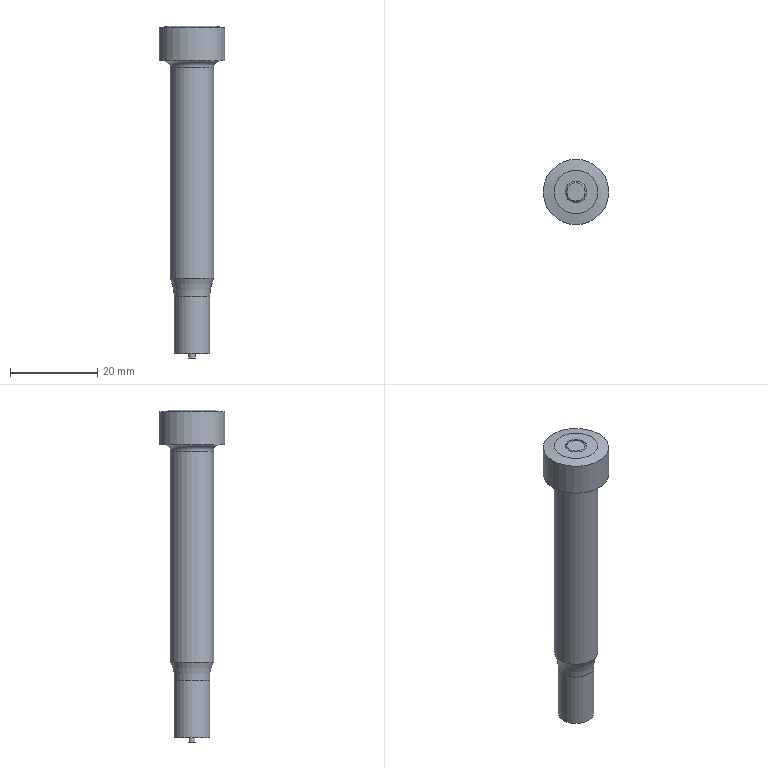Part | NX | features APJAS10-90-P8.10_2 2 | 1 solid | 20 faces | box 15 x 15 x 76 mm | volume 6168 mm3 | cylinder 8 | plane 7 | torus 2 | cone 2 | spline 1 | commonest cylinder face diameters 1.6 x1 1.8 x1 4.2 x1 4.4 x1 4.9 x1 8.1 x1
STEP:
#1=CARTESIAN_POINT('',(-219.,86.,60.5));
#2=VERTEX_POINT('',#1);
#3=CARTESIAN_POINT('',(-214.,86.,60.5));
#4=DIRECTION('',(0.,0.,1.));
#5=DIRECTION('',(1.,0.,0.));
#6=AXIS2_PLACEMENT_3D('',#3,#4,#5);
#7=CIRCLE('',#6,5.);
#8=EDGE_CURVE('',#2,#2,#7,.T.);
#9=ORIENTED_EDGE('',*,*,#8,.F.);
#10=EDGE_LOOP('',(#9));
#11=FACE_BOUND('',#10,.T.);
#12=CARTESIAN_POINT('',(-209.,86.,12.254));
#13=VERTEX_POINT('',#12);
#14=CARTESIAN_POINT('',(-214.,86.,12.254));
#15=DIRECTION('',(0.,0.,1.));
#16=DIRECTION('',(-1.,0.,0.));
#17=AXIS2_PLACEMENT_3D('',#14,#15,#16);
#18=CIRCLE('',#17,5.);
#19=EDGE_CURVE('',#13,#13,#18,.T.);
#20=ORIENTED_EDGE('',*,*,#19,.T.);
#21=EDGE_LOOP('',(#20));
#22=FACE_BOUND('',#21,.T.);
#23=CARTESIAN_POINT('',(-214.,86.,42.5));
#24=DIRECTION('',(0.,0.,-1.));
#25=DIRECTION('',(1.,0.,0.));
#26=AXIS2_PLACEMENT_3D('',#23,#24,#25);
#27=CYLINDRICAL_SURFACE('',#26,5.);
#28=ADVANCED_FACE('',(#11,#22),#27,.T.);
#29=CARTESIAN_POINT('',(-214.9,86.,23.));
#30=VERTEX_POINT('',#29);
#31=CARTESIAN_POINT('',(-214.,86.,23.));
#32=DIRECTION('',(0.,0.,1.));
#33=DIRECTION('',(-1.,0.,0.));
#34=AXIS2_PLACEMENT_3D('',#31,#32,#33);
#35=CIRCLE('',#34,0.9);
#36=EDGE_CURVE('',#30,#30,#35,.T.);
#37=ORIENTED_EDGE('',*,*,#36,.T.);
#38=EDGE_LOOP('',(#37));
#39=FACE_BOUND('',#38,.T.);
#40=CARTESIAN_POINT('',(-214.9,86.,-5.));
#41=VERTEX_POINT('',#40);
#42=CARTESIAN_POINT('',(-214.,86.,-5.));
#43=DIRECTION('',(0.,0.,1.));
#44=DIRECTION('',(-1.,0.,0.));
#45=AXIS2_PLACEMENT_3D('',#42,#43,#44);
#46=CIRCLE('',#45,0.9);
#47=EDGE_CURVE('',#41,#41,#46,.T.);
#48=ORIENTED_EDGE('',*,*,#47,.F.);
#49=EDGE_LOOP('',(#48));
#50=FACE_BOUND('',#49,.T.);
#51=CARTESIAN_POINT('',(-214.,86.,9.));
#52=DIRECTION('',(0.,0.,-1.));
#53=DIRECTION('',(1.,0.,0.));
#54=AXIS2_PLACEMENT_3D('',#51,#52,#53);
#55=CYLINDRICAL_SURFACE('',#54,0.9);
#56=ADVANCED_FACE('',(#39,#50),#55,.F.);
#57=CARTESIAN_POINT('',(-211.55,86.,69.632));
#58=VERTEX_POINT('',#57);
#59=CARTESIAN_POINT('',(-214.,86.,69.632));
#60=DIRECTION('',(0.,0.,1.));
#61=DIRECTION('',(1.,0.,0.));
#62=AXIS2_PLACEMENT_3D('',#59,#60,#61);
#63=CIRCLE('',#62,2.45);
#64=EDGE_CURVE('',#58,#58,#63,.T.);
#65=ORIENTED_EDGE('',*,*,#64,.F.);
#66=EDGE_LOOP('',(#65));
#67=FACE_BOUND('',#66,.T.);
#68=CARTESIAN_POINT('',(-216.45,86.,70.));
#69=VERTEX_POINT('',#68);
#70=CARTESIAN_POINT('',(-214.,86.,70.));
#71=DIRECTION('',(0.,0.,-1.));
#72=DIRECTION('',(-1.,0.,0.));
#73=AXIS2_PLACEMENT_3D('',#70,#71,#72);
#74=CIRCLE('',#73,2.45);
#75=EDGE_CURVE('',#69,#69,#74,.T.);
#76=ORIENTED_EDGE('',*,*,#75,.F.);
#77=EDGE_LOOP('',(#76));
#78=FACE_BOUND('',#77,.T.);
#79=CARTESIAN_POINT('',(-214.,86.,68.775));
#80=DIRECTION('',(0.,0.,-1.));
#81=DIRECTION('',(1.,0.,0.));
#82=AXIS2_PLACEMENT_3D('',#79,#80,#81);
#83=CYLINDRICAL_SURFACE('',#82,2.45);
#84=ADVANCED_FACE('',(#67,#78),#83,.F.);
#85=ORIENTED_EDGE('',*,*,#8,.T.);
#86=EDGE_LOOP('',(#85));
#87=FACE_BOUND('',#86,.T.);
#88=CARTESIAN_POINT('',(-220.5,86.,62.));
#89=VERTEX_POINT('',#88);
#90=CARTESIAN_POINT('',(-214.,86.,62.));
#91=DIRECTION('',(0.,0.,-1.));
#92=DIRECTION('',(1.,0.,0.));
#93=AXIS2_PLACEMENT_3D('',#90,#91,#92);
#94=CIRCLE('',#93,6.5);
#95=EDGE_CURVE('',#89,#89,#94,.T.);
#96=ORIENTED_EDGE('',*,*,#95,.T.);
#97=EDGE_LOOP('',(#96));
#98=FACE_BOUND('',#97,.T.);
#99=CARTESIAN_POINT('',(-214.,86.,60.5));
#100=DIRECTION('',(0.,0.,1.));
#101=DIRECTION('',(-1.,0.,0.));
#102=AXIS2_PLACEMENT_3D('',#99,#100,#101);
#103=TOROIDAL_SURFACE('',#102,6.5,1.5);
#104=ADVANCED_FACE('',(#87,#98),#103,.F.);
#105=CARTESIAN_POINT('',(-221.5,86.,62.));
#106=VERTEX_POINT('',#105);
#107=CARTESIAN_POINT('',(-214.,86.,62.));
#108=DIRECTION('',(0.,0.,-1.));
#109=DIRECTION('',(-1.,0.,0.));
#110=AXIS2_PLACEMENT_3D('',#107,#108,#109);
#111=CIRCLE('',#110,7.5);
#112=EDGE_CURVE('',#106,#106,#111,.T.);
#113=ORIENTED_EDGE('',*,*,#112,.T.);
#114=EDGE_LOOP('',(#113));
#115=FACE_BOUND('',#114,.T.);
#116=ORIENTED_EDGE('',*,*,#95,.F.);
#117=EDGE_LOOP('',(#116));
#118=FACE_BOUND('',#117,.T.);
#119=CARTESIAN_POINT('',(-214.,86.,62.));
#120=DIRECTION('',(0.,0.,-1.));
#121=DIRECTION('',(1.,0.,0.));
#122=AXIS2_PLACEMENT_3D('',#119,#120,#121);
#123=PLANE('',#122);
#124=ADVANCED_FACE('',(#115,#118),#123,.T.);
#125=CARTESIAN_POINT('',(-218.05,86.,8.));
#126=VERTEX_POINT('',#125);
#127=CARTESIAN_POINT('',(-214.,86.,8.));
#128=DIRECTION('',(0.,0.,1.));
#129=DIRECTION('',(-1.,0.,0.));
#130=AXIS2_PLACEMENT_3D('',#127,#128,#129);
#131=CIRCLE('',#130,4.05);
#132=EDGE_CURVE('',#126,#126,#131,.T.);
#133=ORIENTED_EDGE('',*,*,#132,.T.);
#134=EDGE_LOOP('',(#133));
#135=FACE_BOUND('',#134,.T.);
#136=ORIENTED_EDGE('',*,*,#19,.F.);
#137=EDGE_LOOP('',(#136));
#138=FACE_BOUND('',#137,.T.);
#139=CARTESIAN_POINT('',(-214.,86.,8.));
#140=DIRECTION('',(0.,0.,-1.));
#141=DIRECTION('',(1.,0.,0.));
#142=AXIS2_PLACEMENT_3D('',#139,#140,#141);
#143=TOROIDAL_SURFACE('',#142,14.05,10.);
#144=ADVANCED_FACE('',(#135,#138),#143,.F.);
#145=CARTESIAN_POINT('',(-221.5,86.,69.559));
#146=VERTEX_POINT('',#145);
#147=CARTESIAN_POINT('',(-214.,86.,69.559));
#148=DIRECTION('',(0.,0.,1.));
#149=DIRECTION('',(1.,0.,0.));
#150=AXIS2_PLACEMENT_3D('',#147,#148,#149);
#151=CIRCLE('',#150,7.5);
#152=EDGE_CURVE('',#146,#146,#151,.T.);
#153=ORIENTED_EDGE('',*,*,#152,.T.);
#154=EDGE_LOOP('',(#153));
#155=FACE_BOUND('',#154,.T.);
#156=CARTESIAN_POINT('',(-219.,86.,70.));
#157=VERTEX_POINT('',#156);
#158=CARTESIAN_POINT('',(-214.,86.,70.));
#159=DIRECTION('',(0.,0.,-1.));
#160=DIRECTION('',(1.,0.,0.));
#161=AXIS2_PLACEMENT_3D('',#158,#159,#160);
#162=CIRCLE('',#161,5.);
#163=EDGE_CURVE('',#157,#157,#162,.T.);
#164=ORIENTED_EDGE('',*,*,#163,.T.);
#165=EDGE_LOOP('',(#164));
#166=FACE_BOUND('',#165,.T.);
#167=CARTESIAN_POINT('',(-214.,86.,70.));
#168=DIRECTION('',(0.,0.,-1.));
#169=DIRECTION('',(-1.,0.,0.));
#170=AXIS2_PLACEMENT_3D('',#167,#168,#169);
#171=CONICAL_SURFACE('',#170,5.,1.396);
#172=ADVANCED_FACE('',(#155,#166),#171,.T.);
#173=ORIENTED_EDGE('',*,*,#112,.F.);
#174=EDGE_LOOP('',(#173));
#175=FACE_BOUND('',#174,.T.);
#176=ORIENTED_EDGE('',*,*,#152,.F.);
#177=EDGE_LOOP('',(#176));
#178=FACE_BOUND('',#177,.T.);
#179=CARTESIAN_POINT('',(-214.,86.,66.));
#180=DIRECTION('',(0.,0.,-1.));
#181=DIRECTION('',(1.,0.,0.));
#182=AXIS2_PLACEMENT_3D('',#179,#180,#181);
#183=CYLINDRICAL_SURFACE('',#182,7.5);
#184=ADVANCED_FACE('',(#175,#178),#183,.T.);
#185=ORIENTED_EDGE('',*,*,#75,.T.);
#186=EDGE_LOOP('',(#185));
#187=FACE_BOUND('',#186,.T.);
#188=ORIENTED_EDGE('',*,*,#163,.F.);
#189=EDGE_LOOP('',(#188));
#190=FACE_BOUND('',#189,.T.);
#191=CARTESIAN_POINT('',(-214.,86.,70.));
#192=DIRECTION('',(0.,0.,1.));
#193=DIRECTION('',(-1.,0.,0.));
#194=AXIS2_PLACEMENT_3D('',#191,#192,#193);
#195=PLANE('',#194);
#196=ADVANCED_FACE('',(#187,#190),#195,.T.);
#197=ORIENTED_EDGE('',*,*,#132,.F.);
#198=EDGE_LOOP('',(#197));
#199=FACE_BOUND('',#198,.T.);
#200=CARTESIAN_POINT('',(-218.05,86.,-5.));
#201=VERTEX_POINT('',#200);
#202=CARTESIAN_POINT('',(-214.,86.,-5.));
#203=DIRECTION('',(0.,0.,-1.));
#204=DIRECTION('',(-1.,0.,0.));
#205=AXIS2_PLACEMENT_3D('',#202,#203,#204);
#206=CIRCLE('',#205,4.05);
#207=EDGE_CURVE('',#201,#201,#206,.T.);
#208=ORIENTED_EDGE('',*,*,#207,.F.);
#209=EDGE_LOOP('',(#208));
#210=FACE_BOUND('',#209,.T.);
#211=CARTESIAN_POINT('',(-214.,86.,1.5));
#212=DIRECTION('',(0.,0.,-1.));
#213=DIRECTION('',(1.,0.,0.));
#214=AXIS2_PLACEMENT_3D('',#211,#212,#213);
#215=CYLINDRICAL_SURFACE('',#214,4.05);
#216=ADVANCED_FACE('',(#199,#210),#215,.T.);
#217=ORIENTED_EDGE('',*,*,#47,.T.);
#218=EDGE_LOOP('',(#217));
#219=FACE_BOUND('',#218,.T.);
#220=ORIENTED_EDGE('',*,*,#207,.T.);
#221=EDGE_LOOP('',(#220));
#222=FACE_BOUND('',#221,.T.);
#223=CARTESIAN_POINT('',(-214.,86.,-5.));
#224=DIRECTION('',(0.,0.,-1.));
#225=DIRECTION('',(1.,0.,0.));
#226=AXIS2_PLACEMENT_3D('',#223,#224,#225);
#227=PLANE('',#226);
#228=ADVANCED_FACE('',(#219,#222),#227,.T.);
#229=CARTESIAN_POINT('',(-211.917,86.,70.));
#230=VERTEX_POINT('',#229);
#231=CARTESIAN_POINT('',(-214.,86.,70.));
#232=DIRECTION('',(0.,0.,-1.));
#233=DIRECTION('',(1.,0.,0.));
#234=AXIS2_PLACEMENT_3D('',#231,#232,#233);
#235=CIRCLE('',#234,2.083);
#236=EDGE_CURVE('',#230,#230,#235,.T.);
#237=ORIENTED_EDGE('',*,*,#236,.F.);
#238=EDGE_LOOP('',(#237));
#239=FACE_BOUND('',#238,.T.);
#240=CARTESIAN_POINT('',(-214.,86.,70.));
#241=DIRECTION('',(0.,0.,1.));
#242=DIRECTION('',(-1.,0.,0.));
#243=AXIS2_PLACEMENT_3D('',#240,#241,#242);
#244=PLANE('',#243);
#245=ADVANCED_FACE('',(#239),#244,.T.);
#246=ORIENTED_EDGE('',*,*,#64,.T.);
#247=EDGE_LOOP('',(#246));
#248=FACE_BOUND('',#247,.T.);
#249=ORIENTED_EDGE('',*,*,#236,.T.);
#250=EDGE_LOOP('',(#249));
#251=FACE_BOUND('',#250,.T.);
#252=CARTESIAN_POINT('',(-214.,86.,70.));
#253=DIRECTION('',(0.,0.,-1.));
#254=DIRECTION('',(-1.,0.,0.));
#255=AXIS2_PLACEMENT_3D('',#252,#253,#254);
#256=CONICAL_SURFACE('',#255,2.083,0.7854);
#257=ADVANCED_FACE('',(#248,#251),#256,.T.);
#258=CARTESIAN_POINT('',(-214.8,86.,23.));
#259=VERTEX_POINT('',#258);
#260=CARTESIAN_POINT('',(-214.,86.,23.));
#261=DIRECTION('',(0.,0.,-1.));
#262=DIRECTION('',(-1.,0.,0.));
#263=AXIS2_PLACEMENT_3D('',#260,#261,#262);
#264=CIRCLE('',#263,0.8);
#265=EDGE_CURVE('',#259,#259,#264,.F.);
#266=ORIENTED_EDGE('',*,*,#265,.T.);
#267=EDGE_LOOP('',(#266));
#268=FACE_BOUND('',#267,.T.);
#269=ORIENTED_EDGE('',*,*,#36,.F.);
#270=EDGE_LOOP('',(#269));
#271=FACE_BOUND('',#270,.T.);
#272=CARTESIAN_POINT('',(-214.,86.,23.));
#273=DIRECTION('',(0.,0.,-1.));
#274=DIRECTION('',(1.,0.,0.));
#275=AXIS2_PLACEMENT_3D('',#272,#273,#274);
#276=PLANE('',#275);
#277=ADVANCED_FACE('',(#268,#271),#276,.T.);
#278=ORIENTED_EDGE('',*,*,#265,.F.);
#279=EDGE_LOOP('',(#278));
#280=FACE_BOUND('',#279,.T.);
#281=CARTESIAN_POINT('',(-214.8,86.,-6.));
#282=VERTEX_POINT('',#281);
#283=CARTESIAN_POINT('',(-214.,86.,-6.));
#284=DIRECTION('',(0.,0.,-1.));
#285=DIRECTION('',(-1.,0.,0.));
#286=AXIS2_PLACEMENT_3D('',#283,#284,#285);
#287=CIRCLE('',#286,0.8);
#288=EDGE_CURVE('',#282,#282,#287,.T.);
#289=ORIENTED_EDGE('',*,*,#288,.F.);
#290=EDGE_LOOP('',(#289));
#291=FACE_BOUND('',#290,.T.);
#292=CARTESIAN_POINT('',(-214.,86.,8.5));
#293=DIRECTION('',(0.,0.,-1.));
#294=DIRECTION('',(1.,0.,0.));
#295=AXIS2_PLACEMENT_3D('',#292,#293,#294);
#296=CYLINDRICAL_SURFACE('',#295,0.8);
#297=ADVANCED_FACE('',(#280,#291),#296,.T.);
#298=ORIENTED_EDGE('',*,*,#288,.T.);
#299=EDGE_LOOP('',(#298));
#300=FACE_BOUND('',#299,.T.);
#301=CARTESIAN_POINT('',(-214.,86.,-6.));
#302=DIRECTION('',(0.,0.,-1.));
#303=DIRECTION('',(1.,0.,0.));
#304=AXIS2_PLACEMENT_3D('',#301,#302,#303);
#305=PLANE('',#304);
#306=ADVANCED_FACE('',(#300),#305,.T.);
#307=CLOSED_SHELL('',(#28,#56,#84,#104,#124,#144,#172,#184,#196,#216,#228,#245,#257,#277,#297,#306));
#308=CARTESIAN_POINT('',(-211.8,86.002,65.1));
#309=VERTEX_POINT('',#308);
#310=CARTESIAN_POINT('',(-212.276,84.276,65.1));
#311=CARTESIAN_POINT('',(-211.561,86.002,65.1));
#312=CARTESIAN_POINT('',(-212.279,87.727,65.1));
#313=CARTESIAN_POINT('',(-214.001,88.438,65.1));
#314=CARTESIAN_POINT('',(-215.727,87.722,65.1));
#315=CARTESIAN_POINT('',(-216.437,85.998,65.1));
#316=CARTESIAN_POINT('',(-215.724,84.276,65.1));
#317=CARTESIAN_POINT('',(-213.998,83.562,65.1));
#318=CARTESIAN_POINT('',(-212.276,84.276,65.1));
#319=CARTESIAN_POINT('',(-211.561,86.002,65.1));
#320=CARTESIAN_POINT('',(-212.279,87.727,65.1));
#321=B_SPLINE_CURVE_WITH_KNOTS('',3,(#310,#311,#312,#313,#314,#315,#316,#317,#318,#319,#320),.UNSPECIFIED.,.T.,.F.,(1,1,1,1,1,1,1,1,1,1,1,1,1,1,1),(-0.00518,-0.003453,-0.001727,0.,0.001727,0.003453,0.00518,0.006907,0.008633,0.01036,0.01209,0.01381,0.01554,0.01727,0.01899),.UNSPECIFIED.);
#322=EDGE_CURVE('',#309,#309,#321,.T.);
#323=ORIENTED_EDGE('',*,*,#322,.T.);
#324=EDGE_LOOP('',(#323));
#325=FACE_BOUND('',#324,.T.);
#326=CARTESIAN_POINT('',(-216.2,86.,23.));
#327=VERTEX_POINT('',#326);
#328=CARTESIAN_POINT('',(-214.,86.,23.));
#329=DIRECTION('',(0.,0.,-1.));
#330=DIRECTION('',(-1.,0.,0.));
#331=AXIS2_PLACEMENT_3D('',#328,#329,#330);
#332=CIRCLE('',#331,2.2);
#333=EDGE_CURVE('',#327,#327,#332,.T.);
#334=ORIENTED_EDGE('',*,*,#333,.T.);
#335=EDGE_LOOP('',(#334));
#336=FACE_BOUND('',#335,.T.);
#337=CARTESIAN_POINT('',(-214.,86.,52.775));
#338=DIRECTION('',(0.,0.,-1.));
#339=DIRECTION('',(1.,0.,0.));
#340=AXIS2_PLACEMENT_3D('',#337,#338,#339);
#341=CYLINDRICAL_SURFACE('',#340,2.2);
#342=ADVANCED_FACE('',(#325,#336),#341,.F.);
#343=CARTESIAN_POINT('',(-216.1,86.,23.));
#344=VERTEX_POINT('',#343);
#345=CARTESIAN_POINT('',(-214.,86.,23.));
#346=DIRECTION('',(0.,0.,-1.));
#347=DIRECTION('',(-1.,0.,0.));
#348=AXIS2_PLACEMENT_3D('',#345,#346,#347);
#349=CIRCLE('',#348,2.1);
#350=EDGE_CURVE('',#344,#344,#349,.T.);
#351=ORIENTED_EDGE('',*,*,#350,.T.);
#352=EDGE_LOOP('',(#351));
#353=FACE_BOUND('',#352,.T.);
#354=ORIENTED_EDGE('',*,*,#333,.F.);
#355=EDGE_LOOP('',(#354));
#356=FACE_BOUND('',#355,.T.);
#357=CARTESIAN_POINT('',(-214.,86.,23.));
#358=DIRECTION('',(0.,0.,-1.));
#359=DIRECTION('',(1.,0.,0.));
#360=AXIS2_PLACEMENT_3D('',#357,#358,#359);
#361=PLANE('',#360);
#362=ADVANCED_FACE('',(#353,#356),#361,.F.);
#363=ORIENTED_EDGE('',*,*,#322,.F.);
#364=CARTESIAN_POINT('',(-211.9,86.002,64.961));
#365=VERTEX_POINT('',#364);
#366=CARTESIAN_POINT('',(-211.55,86.002,65.448));
#367=DIRECTION('',(-0.5832,-0.0004724,-0.8123));
#368=VECTOR('',#367,1000.);
#369=LINE('',#366,#368);
#370=EDGE_CURVE('',#309,#365,#369,.T.);
#371=ORIENTED_EDGE('',*,*,#370,.T.);
#372=CARTESIAN_POINT('',(-211.9,86.,64.961));
#373=VERTEX_POINT('',#372);
#374=CARTESIAN_POINT('',(-211.9,86.002,64.961));
#375=CARTESIAN_POINT('',(-211.9,86.557,64.961));
#376=CARTESIAN_POINT('',(-212.357,87.645,64.961));
#377=CARTESIAN_POINT('',(-214.001,88.328,64.961));
#378=CARTESIAN_POINT('',(-215.647,87.644,64.961));
#379=CARTESIAN_POINT('',(-216.326,85.999,64.961));
#380=CARTESIAN_POINT('',(-215.647,84.356,64.961));
#381=CARTESIAN_POINT('',(-214.,83.672,64.961));
#382=CARTESIAN_POINT('',(-212.356,84.356,64.961));
#383=CARTESIAN_POINT('',(-211.9,85.445,64.961));
#384=CARTESIAN_POINT('',(-211.9,86.,64.961));
#385=B_SPLINE_CURVE_WITH_KNOTS('',3,(#374,#375,#376,#377,#378,#379,#380,#381,#382,#383,#384),.UNSPECIFIED.,.F.,.F.,(4,1,1,1,1,1,1,1,4),(0.,0.001646,0.003293,0.004939,0.006585,0.008232,0.009878,0.01152,0.01317),.UNSPECIFIED.);
#386=EDGE_CURVE('',#365,#373,#385,.T.);
#387=ORIENTED_EDGE('',*,*,#386,.T.);
#388=CARTESIAN_POINT('',(-211.9,86.,64.961));
#389=CARTESIAN_POINT('',(-211.9,86.001,64.961));
#390=CARTESIAN_POINT('',(-211.9,86.001,64.961));
#391=CARTESIAN_POINT('',(-211.9,86.002,64.961));
#392=B_SPLINE_CURVE_WITH_KNOTS('',3,(#388,#389,#390,#391),.UNSPECIFIED.,.F.,.F.,(4,4),(0.003447,0.003449),.UNSPECIFIED.);
#393=EDGE_CURVE('',#373,#365,#392,.T.);
#394=ORIENTED_EDGE('',*,*,#393,.T.);
#395=ORIENTED_EDGE('',*,*,#370,.F.);
#396=EDGE_LOOP('',(#363,#371,#387,#394,#395));
#397=FACE_BOUND('',#396,.T.);
#398=CARTESIAN_POINT('',(-211.901,85.729,64.96));
#399=CARTESIAN_POINT('',(-211.901,85.729,64.96));
#400=CARTESIAN_POINT('',(-211.9,85.729,64.96));
#401=CARTESIAN_POINT('',(-211.9,85.729,64.961));
#402=CARTESIAN_POINT('',(-211.867,85.725,65.006));
#403=CARTESIAN_POINT('',(-211.835,85.721,65.051));
#404=CARTESIAN_POINT('',(-211.803,85.717,65.097));
#405=CARTESIAN_POINT('',(-211.802,85.716,65.098));
#406=CARTESIAN_POINT('',(-211.801,85.716,65.099));
#407=CARTESIAN_POINT('',(-211.8,85.716,65.1));
#408=CARTESIAN_POINT('',(-211.8,85.716,65.101));
#409=CARTESIAN_POINT('',(-211.799,85.716,65.101));
#410=CARTESIAN_POINT('',(-211.799,85.716,65.102));
#411=CARTESIAN_POINT('',(-211.901,86.154,64.96));
#412=CARTESIAN_POINT('',(-211.901,86.154,64.96));
#413=CARTESIAN_POINT('',(-211.9,86.154,64.96));
#414=CARTESIAN_POINT('',(-211.9,86.154,64.961));
#415=CARTESIAN_POINT('',(-211.867,86.157,65.006));
#416=CARTESIAN_POINT('',(-211.835,86.159,65.051));
#417=CARTESIAN_POINT('',(-211.803,86.162,65.097));
#418=CARTESIAN_POINT('',(-211.802,86.162,65.098));
#419=CARTESIAN_POINT('',(-211.801,86.162,65.099));
#420=CARTESIAN_POINT('',(-211.8,86.162,65.1));
#421=CARTESIAN_POINT('',(-211.8,86.162,65.101));
#422=CARTESIAN_POINT('',(-211.799,86.162,65.101));
#423=CARTESIAN_POINT('',(-211.799,86.162,65.102));
#424=CARTESIAN_POINT('',(-211.918,86.31,64.96));
#425=CARTESIAN_POINT('',(-211.918,86.31,64.96));
#426=CARTESIAN_POINT('',(-211.917,86.31,64.96));
#427=CARTESIAN_POINT('',(-211.917,86.31,64.961));
#428=CARTESIAN_POINT('',(-211.885,86.314,65.006));
#429=CARTESIAN_POINT('',(-211.853,86.319,65.051));
#430=CARTESIAN_POINT('',(-211.821,86.324,65.097));
#431=CARTESIAN_POINT('',(-211.82,86.324,65.098));
#432=CARTESIAN_POINT('',(-211.819,86.324,65.099));
#433=CARTESIAN_POINT('',(-211.818,86.324,65.1));
#434=CARTESIAN_POINT('',(-211.818,86.324,65.101));
#435=CARTESIAN_POINT('',(-211.817,86.324,65.101));
#436=CARTESIAN_POINT('',(-211.817,86.325,65.102));
#437=CARTESIAN_POINT('',(-211.986,86.611,64.96));
#438=CARTESIAN_POINT('',(-211.985,86.611,64.96));
#439=CARTESIAN_POINT('',(-211.985,86.611,64.96));
#440=CARTESIAN_POINT('',(-211.985,86.611,64.961));
#441=CARTESIAN_POINT('',(-211.954,86.62,65.006));
#442=CARTESIAN_POINT('',(-211.923,86.63,65.051));
#443=CARTESIAN_POINT('',(-211.891,86.639,65.097));
#444=CARTESIAN_POINT('',(-211.891,86.639,65.098));
#445=CARTESIAN_POINT('',(-211.89,86.64,65.099));
#446=CARTESIAN_POINT('',(-211.889,86.64,65.1));
#447=CARTESIAN_POINT('',(-211.889,86.64,65.101));
#448=CARTESIAN_POINT('',(-211.888,86.64,65.101));
#449=CARTESIAN_POINT('',(-211.888,86.64,65.102));
#450=CARTESIAN_POINT('',(-212.036,86.758,64.96));
#451=CARTESIAN_POINT('',(-212.036,86.758,64.96));
#452=CARTESIAN_POINT('',(-212.036,86.758,64.96));
#453=CARTESIAN_POINT('',(-212.036,86.759,64.961));
#454=CARTESIAN_POINT('',(-212.005,86.77,65.006));
#455=CARTESIAN_POINT('',(-211.975,86.782,65.051));
#456=CARTESIAN_POINT('',(-211.945,86.794,65.097));
#457=CARTESIAN_POINT('',(-211.944,86.794,65.098));
#458=CARTESIAN_POINT('',(-211.943,86.794,65.099));
#459=CARTESIAN_POINT('',(-211.942,86.795,65.1));
#460=CARTESIAN_POINT('',(-211.942,86.795,65.101));
#461=CARTESIAN_POINT('',(-211.941,86.795,65.101));
#462=CARTESIAN_POINT('',(-211.941,86.795,65.102));
#463=CARTESIAN_POINT('',(-212.218,87.143,64.96));
#464=CARTESIAN_POINT('',(-212.218,87.143,64.96));
#465=CARTESIAN_POINT('',(-212.218,87.143,64.96));
#466=CARTESIAN_POINT('',(-212.218,87.143,64.961));
#467=CARTESIAN_POINT('',(-212.19,87.161,65.006));
#468=CARTESIAN_POINT('',(-212.162,87.178,65.051));
#469=CARTESIAN_POINT('',(-212.135,87.196,65.097));
#470=CARTESIAN_POINT('',(-212.134,87.196,65.098));
#471=CARTESIAN_POINT('',(-212.133,87.197,65.099));
#472=CARTESIAN_POINT('',(-212.133,87.197,65.1));
#473=CARTESIAN_POINT('',(-212.132,87.198,65.101));
#474=CARTESIAN_POINT('',(-212.132,87.198,65.101));
#475=CARTESIAN_POINT('',(-212.132,87.198,65.102));
#476=CARTESIAN_POINT('',(-212.385,87.368,64.96));
#477=CARTESIAN_POINT('',(-212.385,87.369,64.96));
#478=CARTESIAN_POINT('',(-212.385,87.369,64.96));
#479=CARTESIAN_POINT('',(-212.385,87.369,64.961));
#480=CARTESIAN_POINT('',(-212.36,87.39,65.006));
#481=CARTESIAN_POINT('',(-212.335,87.411,65.051));
#482=CARTESIAN_POINT('',(-212.31,87.433,65.097));
#483=CARTESIAN_POINT('',(-212.309,87.433,65.098));
#484=CARTESIAN_POINT('',(-212.308,87.434,65.099));
#485=CARTESIAN_POINT('',(-212.308,87.434,65.1));
#486=CARTESIAN_POINT('',(-212.307,87.434,65.101));
#487=CARTESIAN_POINT('',(-212.307,87.435,65.101));
#488=CARTESIAN_POINT('',(-212.307,87.435,65.102));
#489=CARTESIAN_POINT('',(-212.785,87.733,64.96));
#490=CARTESIAN_POINT('',(-212.785,87.734,64.96));
#491=CARTESIAN_POINT('',(-212.785,87.734,64.96));
#492=CARTESIAN_POINT('',(-212.785,87.734,64.961));
#493=CARTESIAN_POINT('',(-212.766,87.761,65.006));
#494=CARTESIAN_POINT('',(-212.747,87.788,65.051));
#495=CARTESIAN_POINT('',(-212.729,87.815,65.097));
#496=CARTESIAN_POINT('',(-212.728,87.815,65.098));
#497=CARTESIAN_POINT('',(-212.728,87.816,65.099));
#498=CARTESIAN_POINT('',(-212.727,87.817,65.1));
#499=CARTESIAN_POINT('',(-212.727,87.817,65.101));
#500=CARTESIAN_POINT('',(-212.727,87.817,65.101));
#501=CARTESIAN_POINT('',(-212.726,87.818,65.102));
#502=CARTESIAN_POINT('',(-213.026,87.879,64.96));
#503=CARTESIAN_POINT('',(-213.026,87.879,64.96));
#504=CARTESIAN_POINT('',(-213.025,87.88,64.96));
#505=CARTESIAN_POINT('',(-213.025,87.88,64.961));
#506=CARTESIAN_POINT('',(-213.01,87.909,65.006));
#507=CARTESIAN_POINT('',(-212.995,87.938,65.051));
#508=CARTESIAN_POINT('',(-212.98,87.967,65.097));
#509=CARTESIAN_POINT('',(-212.98,87.968,65.098));
#510=CARTESIAN_POINT('',(-212.979,87.969,65.099));
#511=CARTESIAN_POINT('',(-212.979,87.969,65.1));
#512=CARTESIAN_POINT('',(-212.979,87.97,65.101));
#513=CARTESIAN_POINT('',(-212.979,87.97,65.101));
#514=CARTESIAN_POINT('',(-212.978,87.97,65.102));
#515=CARTESIAN_POINT('',(-213.534,88.065,64.96));
#516=CARTESIAN_POINT('',(-213.534,88.065,64.96));
#517=CARTESIAN_POINT('',(-213.534,88.065,64.96));
#518=CARTESIAN_POINT('',(-213.534,88.066,64.961));
#519=CARTESIAN_POINT('',(-213.527,88.098,65.006));
#520=CARTESIAN_POINT('',(-213.52,88.129,65.051));
#521=CARTESIAN_POINT('',(-213.513,88.161,65.097));
#522=CARTESIAN_POINT('',(-213.512,88.162,65.098));
#523=CARTESIAN_POINT('',(-213.512,88.163,65.099));
#524=CARTESIAN_POINT('',(-213.512,88.164,65.1));
#525=CARTESIAN_POINT('',(-213.512,88.164,65.101));
#526=CARTESIAN_POINT('',(-213.512,88.165,65.101));
#527=CARTESIAN_POINT('',(-213.512,88.165,65.102));
#528=CARTESIAN_POINT('',(-213.812,88.108,64.96));
#529=CARTESIAN_POINT('',(-213.812,88.108,64.96));
#530=CARTESIAN_POINT('',(-213.812,88.109,64.96));
#531=CARTESIAN_POINT('',(-213.812,88.109,64.961));
#532=CARTESIAN_POINT('',(-213.809,88.142,65.006));
#533=CARTESIAN_POINT('',(-213.806,88.174,65.051));
#534=CARTESIAN_POINT('',(-213.803,88.207,65.097));
#535=CARTESIAN_POINT('',(-213.803,88.208,65.098));
#536=CARTESIAN_POINT('',(-213.803,88.209,65.099));
#537=CARTESIAN_POINT('',(-213.803,88.209,65.1));
#538=CARTESIAN_POINT('',(-213.803,88.21,65.101));
#539=CARTESIAN_POINT('',(-213.803,88.21,65.101));
#540=CARTESIAN_POINT('',(-213.803,88.211,65.102));
#541=CARTESIAN_POINT('',(-214.353,88.087,64.96));
#542=CARTESIAN_POINT('',(-214.353,88.087,64.96));
#543=CARTESIAN_POINT('',(-214.353,88.087,64.96));
#544=CARTESIAN_POINT('',(-214.353,88.088,64.961));
#545=CARTESIAN_POINT('',(-214.359,88.12,65.006));
#546=CARTESIAN_POINT('',(-214.364,88.152,65.051));
#547=CARTESIAN_POINT('',(-214.37,88.185,65.097));
#548=CARTESIAN_POINT('',(-214.37,88.185,65.098));
#549=CARTESIAN_POINT('',(-214.37,88.186,65.099));
#550=CARTESIAN_POINT('',(-214.37,88.187,65.1));
#551=CARTESIAN_POINT('',(-214.37,88.188,65.101));
#552=CARTESIAN_POINT('',(-214.37,88.188,65.101));
#553=CARTESIAN_POINT('',(-214.37,88.188,65.102));
#554=CARTESIAN_POINT('',(-214.627,88.022,64.96));
#555=CARTESIAN_POINT('',(-214.627,88.022,64.96));
#556=CARTESIAN_POINT('',(-214.627,88.022,64.96));
#557=CARTESIAN_POINT('',(-214.627,88.023,64.961));
#558=CARTESIAN_POINT('',(-214.636,88.054,65.006));
#559=CARTESIAN_POINT('',(-214.646,88.085,65.051));
#560=CARTESIAN_POINT('',(-214.656,88.116,65.097));
#561=CARTESIAN_POINT('',(-214.656,88.117,65.098));
#562=CARTESIAN_POINT('',(-214.656,88.118,65.099));
#563=CARTESIAN_POINT('',(-214.657,88.119,65.1));
#564=CARTESIAN_POINT('',(-214.657,88.119,65.101));
#565=CARTESIAN_POINT('',(-214.657,88.12,65.101));
#566=CARTESIAN_POINT('',(-214.657,88.12,65.102));
#567=CARTESIAN_POINT('',(-215.119,87.797,64.96));
#568=CARTESIAN_POINT('',(-215.119,87.797,64.96));
#569=CARTESIAN_POINT('',(-215.119,87.797,64.96));
#570=CARTESIAN_POINT('',(-215.119,87.797,64.961));
#571=CARTESIAN_POINT('',(-215.137,87.825,65.006));
#572=CARTESIAN_POINT('',(-215.154,87.853,65.051));
#573=CARTESIAN_POINT('',(-215.171,87.881,65.097));
#574=CARTESIAN_POINT('',(-215.172,87.881,65.098));
#575=CARTESIAN_POINT('',(-215.172,87.882,65.099));
#576=CARTESIAN_POINT('',(-215.173,87.883,65.1));
#577=CARTESIAN_POINT('',(-215.173,87.883,65.101));
#578=CARTESIAN_POINT('',(-215.173,87.884,65.101));
#579=CARTESIAN_POINT('',(-215.173,87.884,65.102));
#580=CARTESIAN_POINT('',(-215.347,87.633,64.96));
#581=CARTESIAN_POINT('',(-215.347,87.633,64.96));
#582=CARTESIAN_POINT('',(-215.348,87.633,64.96));
#583=CARTESIAN_POINT('',(-215.348,87.633,64.961));
#584=CARTESIAN_POINT('',(-215.369,87.658,65.006));
#585=CARTESIAN_POINT('',(-215.389,87.684,65.051));
#586=CARTESIAN_POINT('',(-215.41,87.709,65.097));
#587=CARTESIAN_POINT('',(-215.411,87.71,65.098));
#588=CARTESIAN_POINT('',(-215.411,87.71,65.099));
#589=CARTESIAN_POINT('',(-215.412,87.711,65.1));
#590=CARTESIAN_POINT('',(-215.412,87.711,65.101));
#591=CARTESIAN_POINT('',(-215.412,87.712,65.101));
#592=CARTESIAN_POINT('',(-215.413,87.712,65.102));
#593=CARTESIAN_POINT('',(-215.717,87.237,64.96));
#594=CARTESIAN_POINT('',(-215.718,87.237,64.96));
#595=CARTESIAN_POINT('',(-215.718,87.238,64.96));
#596=CARTESIAN_POINT('',(-215.718,87.238,64.961));
#597=CARTESIAN_POINT('',(-215.745,87.257,65.006));
#598=CARTESIAN_POINT('',(-215.771,87.276,65.051));
#599=CARTESIAN_POINT('',(-215.798,87.295,65.097));
#600=CARTESIAN_POINT('',(-215.798,87.296,65.098));
#601=CARTESIAN_POINT('',(-215.799,87.296,65.099));
#602=CARTESIAN_POINT('',(-215.8,87.297,65.1));
#603=CARTESIAN_POINT('',(-215.8,87.297,65.101));
#604=CARTESIAN_POINT('',(-215.8,87.297,65.101));
#605=CARTESIAN_POINT('',(-215.801,87.297,65.102));
#606=CARTESIAN_POINT('',(-215.866,86.999,64.96));
#607=CARTESIAN_POINT('',(-215.866,86.999,64.96));
#608=CARTESIAN_POINT('',(-215.867,86.999,64.96));
#609=CARTESIAN_POINT('',(-215.867,86.999,64.961));
#610=CARTESIAN_POINT('',(-215.896,87.015,65.006));
#611=CARTESIAN_POINT('',(-215.925,87.03,65.051));
#612=CARTESIAN_POINT('',(-215.953,87.046,65.097));
#613=CARTESIAN_POINT('',(-215.954,87.046,65.098));
#614=CARTESIAN_POINT('',(-215.955,87.046,65.099));
#615=CARTESIAN_POINT('',(-215.956,87.047,65.1));
#616=CARTESIAN_POINT('',(-215.956,87.047,65.101));
#617=CARTESIAN_POINT('',(-215.956,87.047,65.101));
#618=CARTESIAN_POINT('',(-215.957,87.047,65.102));
#619=CARTESIAN_POINT('',(-216.058,86.493,64.96));
#620=CARTESIAN_POINT('',(-216.059,86.493,64.96));
#621=CARTESIAN_POINT('',(-216.059,86.493,64.96));
#622=CARTESIAN_POINT('',(-216.059,86.493,64.961));
#623=CARTESIAN_POINT('',(-216.091,86.5,65.006));
#624=CARTESIAN_POINT('',(-216.123,86.508,65.051));
#625=CARTESIAN_POINT('',(-216.155,86.516,65.097));
#626=CARTESIAN_POINT('',(-216.156,86.516,65.098));
#627=CARTESIAN_POINT('',(-216.156,86.516,65.099));
#628=CARTESIAN_POINT('',(-216.157,86.516,65.1));
#629=CARTESIAN_POINT('',(-216.158,86.516,65.101));
#630=CARTESIAN_POINT('',(-216.158,86.516,65.101));
#631=CARTESIAN_POINT('',(-216.158,86.517,65.102));
#632=CARTESIAN_POINT('',(-216.106,86.216,64.96));
#633=CARTESIAN_POINT('',(-216.106,86.216,64.96));
#634=CARTESIAN_POINT('',(-216.106,86.216,64.96));
#635=CARTESIAN_POINT('',(-216.106,86.216,64.961));
#636=CARTESIAN_POINT('',(-216.139,86.219,65.006));
#637=CARTESIAN_POINT('',(-216.172,86.222,65.051));
#638=CARTESIAN_POINT('',(-216.204,86.226,65.097));
#639=CARTESIAN_POINT('',(-216.205,86.226,65.098));
#640=CARTESIAN_POINT('',(-216.206,86.226,65.099));
#641=CARTESIAN_POINT('',(-216.207,86.226,65.1));
#642=CARTESIAN_POINT('',(-216.207,86.226,65.101));
#643=CARTESIAN_POINT('',(-216.207,86.226,65.101));
#644=CARTESIAN_POINT('',(-216.208,86.226,65.102));
#645=CARTESIAN_POINT('',(-216.091,85.674,64.96));
#646=CARTESIAN_POINT('',(-216.092,85.674,64.96));
#647=CARTESIAN_POINT('',(-216.092,85.674,64.96));
#648=CARTESIAN_POINT('',(-216.092,85.674,64.961));
#649=CARTESIAN_POINT('',(-216.125,85.669,65.006));
#650=CARTESIAN_POINT('',(-216.157,85.664,65.051));
#651=CARTESIAN_POINT('',(-216.189,85.659,65.097));
#652=CARTESIAN_POINT('',(-216.19,85.659,65.098));
#653=CARTESIAN_POINT('',(-216.191,85.659,65.099));
#654=CARTESIAN_POINT('',(-216.192,85.659,65.1));
#655=CARTESIAN_POINT('',(-216.192,85.659,65.101));
#656=CARTESIAN_POINT('',(-216.193,85.658,65.101));
#657=CARTESIAN_POINT('',(-216.193,85.658,65.102));
#658=CARTESIAN_POINT('',(-216.03,85.4,64.96));
#659=CARTESIAN_POINT('',(-216.03,85.4,64.96));
#660=CARTESIAN_POINT('',(-216.03,85.4,64.96));
#661=CARTESIAN_POINT('',(-216.031,85.4,64.961));
#662=CARTESIAN_POINT('',(-216.062,85.391,65.006));
#663=CARTESIAN_POINT('',(-216.093,85.381,65.051));
#664=CARTESIAN_POINT('',(-216.125,85.372,65.097));
#665=CARTESIAN_POINT('',(-216.126,85.372,65.098));
#666=CARTESIAN_POINT('',(-216.126,85.371,65.099));
#667=CARTESIAN_POINT('',(-216.127,85.371,65.1));
#668=CARTESIAN_POINT('',(-216.128,85.371,65.101));
#669=CARTESIAN_POINT('',(-216.128,85.371,65.101));
#670=CARTESIAN_POINT('',(-216.128,85.371,65.102));
#671=CARTESIAN_POINT('',(-215.811,84.905,64.96));
#672=CARTESIAN_POINT('',(-215.811,84.904,64.96));
#673=CARTESIAN_POINT('',(-215.812,84.904,64.96));
#674=CARTESIAN_POINT('',(-215.812,84.904,64.961));
#675=CARTESIAN_POINT('',(-215.84,84.887,65.006));
#676=CARTESIAN_POINT('',(-215.868,84.87,65.051));
#677=CARTESIAN_POINT('',(-215.896,84.853,65.097));
#678=CARTESIAN_POINT('',(-215.897,84.853,65.098));
#679=CARTESIAN_POINT('',(-215.897,84.852,65.099));
#680=CARTESIAN_POINT('',(-215.898,84.852,65.1));
#681=CARTESIAN_POINT('',(-215.898,84.852,65.101));
#682=CARTESIAN_POINT('',(-215.899,84.852,65.101));
#683=CARTESIAN_POINT('',(-215.899,84.851,65.102));
#684=CARTESIAN_POINT('',(-215.65,84.674,64.96));
#685=CARTESIAN_POINT('',(-215.65,84.674,64.96));
#686=CARTESIAN_POINT('',(-215.65,84.674,64.96));
#687=CARTESIAN_POINT('',(-215.651,84.674,64.961));
#688=CARTESIAN_POINT('',(-215.676,84.653,65.006));
#689=CARTESIAN_POINT('',(-215.702,84.633,65.051));
#690=CARTESIAN_POINT('',(-215.727,84.612,65.097));
#691=CARTESIAN_POINT('',(-215.728,84.612,65.098));
#692=CARTESIAN_POINT('',(-215.729,84.611,65.099));
#693=CARTESIAN_POINT('',(-215.729,84.611,65.1));
#694=CARTESIAN_POINT('',(-215.73,84.61,65.101));
#695=CARTESIAN_POINT('',(-215.73,84.61,65.101));
#696=CARTESIAN_POINT('',(-215.73,84.61,65.102));
#697=CARTESIAN_POINT('',(-215.26,84.299,64.96));
#698=CARTESIAN_POINT('',(-215.26,84.299,64.96));
#699=CARTESIAN_POINT('',(-215.26,84.299,64.96));
#700=CARTESIAN_POINT('',(-215.26,84.298,64.961));
#701=CARTESIAN_POINT('',(-215.28,84.272,65.006));
#702=CARTESIAN_POINT('',(-215.299,84.246,65.051));
#703=CARTESIAN_POINT('',(-215.319,84.219,65.097));
#704=CARTESIAN_POINT('',(-215.319,84.219,65.098));
#705=CARTESIAN_POINT('',(-215.32,84.218,65.099));
#706=CARTESIAN_POINT('',(-215.32,84.217,65.1));
#707=CARTESIAN_POINT('',(-215.32,84.217,65.101));
#708=CARTESIAN_POINT('',(-215.321,84.217,65.101));
#709=CARTESIAN_POINT('',(-215.321,84.216,65.102));
#710=CARTESIAN_POINT('',(-215.023,84.147,64.96));
#711=CARTESIAN_POINT('',(-215.023,84.147,64.96));
#712=CARTESIAN_POINT('',(-215.023,84.147,64.96));
#713=CARTESIAN_POINT('',(-215.024,84.146,64.961));
#714=CARTESIAN_POINT('',(-215.039,84.118,65.006));
#715=CARTESIAN_POINT('',(-215.055,84.089,65.051));
#716=CARTESIAN_POINT('',(-215.071,84.06,65.097));
#717=CARTESIAN_POINT('',(-215.072,84.06,65.098));
#718=CARTESIAN_POINT('',(-215.072,84.059,65.099));
#719=CARTESIAN_POINT('',(-215.072,84.058,65.1));
#720=CARTESIAN_POINT('',(-215.073,84.058,65.101));
#721=CARTESIAN_POINT('',(-215.073,84.058,65.101));
#722=CARTESIAN_POINT('',(-215.073,84.057,65.102));
#723=CARTESIAN_POINT('',(-214.52,83.948,64.96));
#724=CARTESIAN_POINT('',(-214.52,83.948,64.96));
#725=CARTESIAN_POINT('',(-214.52,83.948,64.96));
#726=CARTESIAN_POINT('',(-214.52,83.947,64.961));
#727=CARTESIAN_POINT('',(-214.528,83.916,65.006));
#728=CARTESIAN_POINT('',(-214.536,83.884,65.051));
#729=CARTESIAN_POINT('',(-214.544,83.852,65.097));
#730=CARTESIAN_POINT('',(-214.544,83.851,65.098));
#731=CARTESIAN_POINT('',(-214.544,83.85,65.099));
#732=CARTESIAN_POINT('',(-214.545,83.85,65.1));
#733=CARTESIAN_POINT('',(-214.545,83.849,65.101));
#734=CARTESIAN_POINT('',(-214.545,83.849,65.101));
#735=CARTESIAN_POINT('',(-214.545,83.848,65.102));
#736=CARTESIAN_POINT('',(-214.243,83.897,64.96));
#737=CARTESIAN_POINT('',(-214.243,83.897,64.96));
#738=CARTESIAN_POINT('',(-214.243,83.897,64.96));
#739=CARTESIAN_POINT('',(-214.243,83.897,64.961));
#740=CARTESIAN_POINT('',(-214.247,83.864,65.006));
#741=CARTESIAN_POINT('',(-214.251,83.832,65.051));
#742=CARTESIAN_POINT('',(-214.255,83.799,65.097));
#743=CARTESIAN_POINT('',(-214.255,83.798,65.098));
#744=CARTESIAN_POINT('',(-214.255,83.797,65.099));
#745=CARTESIAN_POINT('',(-214.255,83.796,65.1));
#746=CARTESIAN_POINT('',(-214.255,83.796,65.101));
#747=CARTESIAN_POINT('',(-214.255,83.796,65.101));
#748=CARTESIAN_POINT('',(-214.255,83.795,65.102));
#749=CARTESIAN_POINT('',(-213.702,83.905,64.96));
#750=CARTESIAN_POINT('',(-213.702,83.904,64.96));
#751=CARTESIAN_POINT('',(-213.702,83.904,64.96));
#752=CARTESIAN_POINT('',(-213.702,83.904,64.961));
#753=CARTESIAN_POINT('',(-213.697,83.871,65.006));
#754=CARTESIAN_POINT('',(-213.692,83.839,65.051));
#755=CARTESIAN_POINT('',(-213.688,83.806,65.097));
#756=CARTESIAN_POINT('',(-213.688,83.806,65.098));
#757=CARTESIAN_POINT('',(-213.688,83.805,65.099));
#758=CARTESIAN_POINT('',(-213.687,83.804,65.1));
#759=CARTESIAN_POINT('',(-213.687,83.804,65.101));
#760=CARTESIAN_POINT('',(-213.687,83.803,65.101));
#761=CARTESIAN_POINT('',(-213.687,83.803,65.102));
#762=CARTESIAN_POINT('',(-213.427,83.963,64.96));
#763=CARTESIAN_POINT('',(-213.427,83.962,64.96));
#764=CARTESIAN_POINT('',(-213.427,83.962,64.96));
#765=CARTESIAN_POINT('',(-213.427,83.962,64.961));
#766=CARTESIAN_POINT('',(-213.418,83.93,65.006));
#767=CARTESIAN_POINT('',(-213.409,83.899,65.051));
#768=CARTESIAN_POINT('',(-213.4,83.867,65.097));
#769=CARTESIAN_POINT('',(-213.4,83.866,65.098));
#770=CARTESIAN_POINT('',(-213.399,83.865,65.099));
#771=CARTESIAN_POINT('',(-213.399,83.865,65.1));
#772=CARTESIAN_POINT('',(-213.399,83.864,65.101));
#773=CARTESIAN_POINT('',(-213.399,83.864,65.101));
#774=CARTESIAN_POINT('',(-213.399,83.864,65.102));
#775=CARTESIAN_POINT('',(-212.929,84.175,64.96));
#776=CARTESIAN_POINT('',(-212.928,84.174,64.96));
#777=CARTESIAN_POINT('',(-212.928,84.174,64.96));
#778=CARTESIAN_POINT('',(-212.928,84.174,64.961));
#779=CARTESIAN_POINT('',(-212.911,84.146,65.006));
#780=CARTESIAN_POINT('',(-212.895,84.117,65.051));
#781=CARTESIAN_POINT('',(-212.878,84.089,65.097));
#782=CARTESIAN_POINT('',(-212.878,84.088,65.098));
#783=CARTESIAN_POINT('',(-212.877,84.088,65.099));
#784=CARTESIAN_POINT('',(-212.877,84.087,65.1));
#785=CARTESIAN_POINT('',(-212.877,84.087,65.101));
#786=CARTESIAN_POINT('',(-212.877,84.086,65.101));
#787=CARTESIAN_POINT('',(-212.876,84.086,65.102));
#788=CARTESIAN_POINT('',(-212.696,84.333,64.96));
#789=CARTESIAN_POINT('',(-212.696,84.332,64.96));
#790=CARTESIAN_POINT('',(-212.696,84.332,64.96));
#791=CARTESIAN_POINT('',(-212.696,84.332,64.961));
#792=CARTESIAN_POINT('',(-212.675,84.306,65.006));
#793=CARTESIAN_POINT('',(-212.655,84.28,65.051));
#794=CARTESIAN_POINT('',(-212.635,84.255,65.097));
#795=CARTESIAN_POINT('',(-212.635,84.254,65.098));
#796=CARTESIAN_POINT('',(-212.634,84.253,65.099));
#797=CARTESIAN_POINT('',(-212.634,84.253,65.1));
#798=CARTESIAN_POINT('',(-212.633,84.252,65.101));
#799=CARTESIAN_POINT('',(-212.633,84.252,65.101));
#800=CARTESIAN_POINT('',(-212.633,84.252,65.102));
#801=CARTESIAN_POINT('',(-212.316,84.718,64.96));
#802=CARTESIAN_POINT('',(-212.316,84.718,64.96));
#803=CARTESIAN_POINT('',(-212.315,84.718,64.96));
#804=CARTESIAN_POINT('',(-212.315,84.718,64.961));
#805=CARTESIAN_POINT('',(-212.289,84.698,65.006));
#806=CARTESIAN_POINT('',(-212.263,84.678,65.051));
#807=CARTESIAN_POINT('',(-212.237,84.658,65.097));
#808=CARTESIAN_POINT('',(-212.236,84.658,65.098));
#809=CARTESIAN_POINT('',(-212.236,84.657,65.099));
#810=CARTESIAN_POINT('',(-212.235,84.657,65.1));
#811=CARTESIAN_POINT('',(-212.235,84.656,65.101));
#812=CARTESIAN_POINT('',(-212.234,84.656,65.101));
#813=CARTESIAN_POINT('',(-212.234,84.656,65.102));
#814=CARTESIAN_POINT('',(-212.161,84.953,64.96));
#815=CARTESIAN_POINT('',(-212.161,84.952,64.96));
#816=CARTESIAN_POINT('',(-212.16,84.952,64.96));
#817=CARTESIAN_POINT('',(-212.16,84.952,64.961));
#818=CARTESIAN_POINT('',(-212.132,84.936,65.006));
#819=CARTESIAN_POINT('',(-212.103,84.92,65.051));
#820=CARTESIAN_POINT('',(-212.075,84.903,65.097));
#821=CARTESIAN_POINT('',(-212.074,84.903,65.098));
#822=CARTESIAN_POINT('',(-212.073,84.903,65.099));
#823=CARTESIAN_POINT('',(-212.072,84.902,65.1));
#824=CARTESIAN_POINT('',(-212.072,84.902,65.101));
#825=CARTESIAN_POINT('',(-212.072,84.902,65.101));
#826=CARTESIAN_POINT('',(-212.071,84.902,65.102));
#827=CARTESIAN_POINT('',(-211.955,85.454,64.96));
#828=CARTESIAN_POINT('',(-211.955,85.453,64.96));
#829=CARTESIAN_POINT('',(-211.955,85.453,64.96));
#830=CARTESIAN_POINT('',(-211.954,85.453,64.961));
#831=CARTESIAN_POINT('',(-211.923,85.445,65.006));
#832=CARTESIAN_POINT('',(-211.891,85.436,65.051));
#833=CARTESIAN_POINT('',(-211.859,85.428,65.097));
#834=CARTESIAN_POINT('',(-211.859,85.428,65.098));
#835=CARTESIAN_POINT('',(-211.858,85.428,65.099));
#836=CARTESIAN_POINT('',(-211.857,85.427,65.1));
#837=CARTESIAN_POINT('',(-211.857,85.427,65.101));
#838=CARTESIAN_POINT('',(-211.856,85.427,65.101));
#839=CARTESIAN_POINT('',(-211.856,85.427,65.102));
#840=CARTESIAN_POINT('',(-211.901,85.729,64.96));
#841=CARTESIAN_POINT('',(-211.901,85.729,64.96));
#842=CARTESIAN_POINT('',(-211.9,85.729,64.96));
#843=CARTESIAN_POINT('',(-211.9,85.729,64.961));
#844=CARTESIAN_POINT('',(-211.867,85.725,65.006));
#845=CARTESIAN_POINT('',(-211.835,85.721,65.051));
#846=CARTESIAN_POINT('',(-211.803,85.717,65.097));
#847=CARTESIAN_POINT('',(-211.802,85.716,65.098));
#848=CARTESIAN_POINT('',(-211.801,85.716,65.099));
#849=CARTESIAN_POINT('',(-211.8,85.716,65.1));
#850=CARTESIAN_POINT('',(-211.8,85.716,65.101));
#851=CARTESIAN_POINT('',(-211.799,85.716,65.101));
#852=CARTESIAN_POINT('',(-211.799,85.716,65.102));
#853=CARTESIAN_POINT('',(-211.901,86.154,64.96));
#854=CARTESIAN_POINT('',(-211.901,86.154,64.96));
#855=CARTESIAN_POINT('',(-211.9,86.154,64.96));
#856=CARTESIAN_POINT('',(-211.9,86.154,64.961));
#857=CARTESIAN_POINT('',(-211.867,86.157,65.006));
#858=CARTESIAN_POINT('',(-211.835,86.159,65.051));
#859=CARTESIAN_POINT('',(-211.803,86.162,65.097));
#860=CARTESIAN_POINT('',(-211.802,86.162,65.098));
#861=CARTESIAN_POINT('',(-211.801,86.162,65.099));
#862=CARTESIAN_POINT('',(-211.8,86.162,65.1));
#863=CARTESIAN_POINT('',(-211.8,86.162,65.101));
#864=CARTESIAN_POINT('',(-211.799,86.162,65.101));
#865=CARTESIAN_POINT('',(-211.799,86.162,65.102));
#866=B_SPLINE_SURFACE_WITH_KNOTS('',3,3,((#398,#399,#400,#401,#402,#403,#404,#405,#406,#407,#408,#409,#410),(#411,#412,#413,#414,#415,#416,#417,#418,#419,#420,#421,#422,#423),(#424,#425,#426,#427,#428,#429,#430,#431,#432,#433,#434,#435,#436),(#437,#438,#439,#440,#441,#442,#443,#444,#445,#446,#447,#448,#449),(#450,#451,#452,#453,#454,#455,#456,#457,#458,#459,#460,#461,#462),(#463,#464,#465,#466,#467,#468,#469,#470,#471,#472,#473,#474,#475),(#476,#477,#478,#479,#480,#481,#482,#483,#484,#485,#486,#487,#488),(#489,#490,#491,#492,#493,#494,#495,#496,#497,#498,#499,#500,#501),(#502,#503,#504,#505,#506,#507,#508,#509,#510,#511,#512,#513,#514),(#515,#516,#517,#518,#519,#520,#521,#522,#523,#524,#525,#526,#527),(#528,#529,#530,#531,#532,#533,#534,#535,#536,#537,#538,#539,#540),(#541,#542,#543,#544,#545,#546,#547,#548,#549,#550,#551,#552,#553),(#554,#555,#556,#557,#558,#559,#560,#561,#562,#563,#564,#565,#566),(#567,#568,#569,#570,#571,#572,#573,#574,#575,#576,#577,#578,#579),(#580,#581,#582,#583,#584,#585,#586,#587,#588,#589,#590,#591,#592),(#593,#594,#595,#596,#597,#598,#599,#600,#601,#602,#603,#604,#605),(#606,#607,#608,#609,#610,#611,#612,#613,#614,#615,#616,#617,#618),(#619,#620,#621,#622,#623,#624,#625,#626,#627,#628,#629,#630,#631),(#632,#633,#634,#635,#636,#637,#638,#639,#640,#641,#642,#643,#644),(#645,#646,#647,#648,#649,#650,#651,#652,#653,#654,#655,#656,#657),(#658,#659,#660,#661,#662,#663,#664,#665,#666,#667,#668,#669,#670),(#671,#672,#673,#674,#675,#676,#677,#678,#679,#680,#681,#682,#683),(#684,#685,#686,#687,#688,#689,#690,#691,#692,#693,#694,#695,#696),(#697,#698,#699,#700,#701,#702,#703,#704,#705,#706,#707,#708,#709),(#710,#711,#712,#713,#714,#715,#716,#717,#718,#719,#720,#721,#722),(#723,#724,#725,#726,#727,#728,#729,#730,#731,#732,#733,#734,#735),(#736,#737,#738,#739,#740,#741,#742,#743,#744,#745,#746,#747,#748),(#749,#750,#751,#752,#753,#754,#755,#756,#757,#758,#759,#760,#761),(#762,#763,#764,#765,#766,#767,#768,#769,#770,#771,#772,#773,#774),(#775,#776,#777,#778,#779,#780,#781,#782,#783,#784,#785,#786,#787),(#788,#789,#790,#791,#792,#793,#794,#795,#796,#797,#798,#799,#800),(#801,#802,#803,#804,#805,#806,#807,#808,#809,#810,#811,#812,#813),(#814,#815,#816,#817,#818,#819,#820,#821,#822,#823,#824,#825,#826),(#827,#828,#829,#830,#831,#832,#833,#834,#835,#836,#837,#838,#839),(#840,#841,#842,#843,#844,#845,#846,#847,#848,#849,#850,#851,#852),(#853,#854,#855,#856,#857,#858,#859,#860,#861,#862,#863,#864,#865)),.RULED_SURF.,.T.,.F.,.F.,(2,2,2,2,2,2,2,2,2,2,2,2,2,2,2,2,2,2,2,2),(4,3,3,3,4),(-0.06196,0.,0.03531,0.07061,0.1326,0.1945,0.2565,0.3184,0.3804,0.4424,0.5043,0.5663,0.6282,0.6902,0.7522,0.8141,0.8761,0.938,1.,1.035),(-0.4033,-0.4,-0.01,0.,0.004738),.UNSPECIFIED.);
#867=ADVANCED_FACE('',(#397),#866,.T.);
#868=ORIENTED_EDGE('',*,*,#393,.F.);
#869=ORIENTED_EDGE('',*,*,#386,.F.);
#870=EDGE_LOOP('',(#868,#869));
#871=FACE_BOUND('',#870,.T.);
#872=ORIENTED_EDGE('',*,*,#350,.F.);
#873=EDGE_LOOP('',(#872));
#874=FACE_BOUND('',#873,.T.);
#875=CARTESIAN_POINT('',(-214.,86.,51.55));
#876=DIRECTION('',(0.,0.,-1.));
#877=DIRECTION('',(1.,0.,0.));
#878=AXIS2_PLACEMENT_3D('',#875,#876,#877);
#879=CYLINDRICAL_SURFACE('',#878,2.1);
#880=ADVANCED_FACE('',(#871,#874),#879,.T.);
#881=CLOSED_SHELL('',(#342,#362,#867,#880));
#882=ORIENTED_CLOSED_SHELL('',*,#881,.F.);
#883=BREP_WITH_VOIDS('',#307,(#882));
#884=(LENGTH_UNIT()NAMED_UNIT(*)SI_UNIT(.MILLI.,.METRE.));
#885=UNCERTAINTY_MEASURE_WITH_UNIT(LENGTH_MEASURE(0.0508),#884,'','');
#886=(NAMED_UNIT(*)PLANE_ANGLE_UNIT()SI_UNIT($,.RADIAN.));
#887=(NAMED_UNIT(*)SI_UNIT($,.STERADIAN.)SOLID_ANGLE_UNIT());
#888=(GEOMETRIC_REPRESENTATION_CONTEXT(3)GLOBAL_UNCERTAINTY_ASSIGNED_CONTEXT((#885))GLOBAL_UNIT_ASSIGNED_CONTEXT((#884,#886,#887))REPRESENTATION_CONTEXT('',''));
#889=ADVANCED_BREP_SHAPE_REPRESENTATION('',(#883),#888);